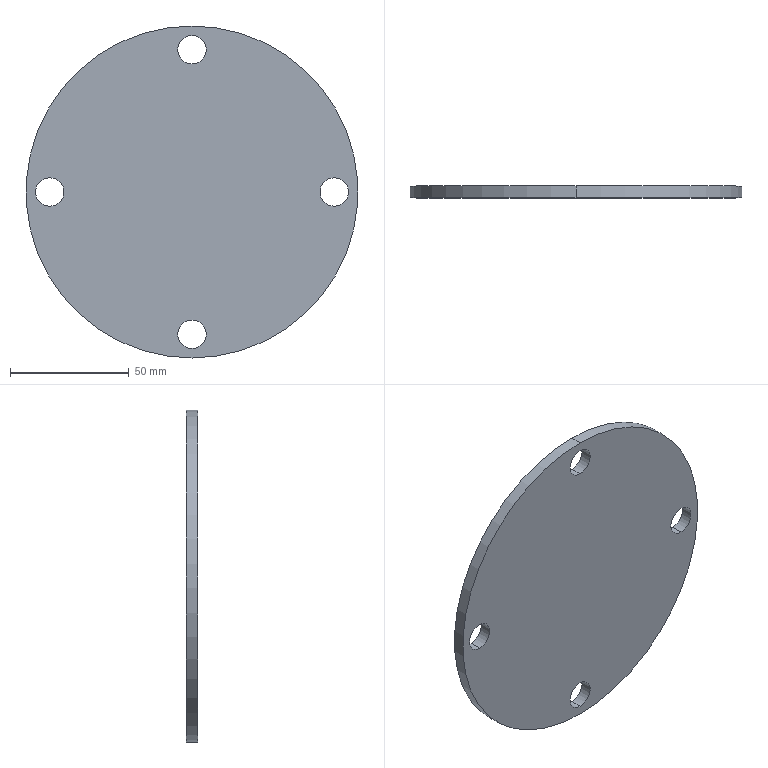Part | SolidWorks | features MirrorStock 1 | 1 solid | 12 faces | box 140 x 5 x 140 mm | volume 74707 mm3 | cylinder 10 | plane 2 | commonest cylinder face diameters 12 x8 140 x2
STEP:
#1=CARTESIAN_POINT('',(0.,0.,54.));
#2=VERTEX_POINT('',#1);
#3=CARTESIAN_POINT('',(0.,0.,66.));
#4=VERTEX_POINT('',#3);
#5=CARTESIAN_POINT('',(0.,0.,60.));
#6=DIRECTION('',(0.,-1.,0.));
#7=DIRECTION('',(0.,0.,-1.));
#8=AXIS2_PLACEMENT_3D('',#5,#6,#7);
#9=CIRCLE('',#8,6.);
#10=EDGE_CURVE('',#2,#4,#9,.T.);
#11=ORIENTED_EDGE('',*,*,#10,.T.);
#12=CARTESIAN_POINT('',(0.,5.,66.));
#13=VERTEX_POINT('',#12);
#14=CARTESIAN_POINT('',(0.,0.,66.));
#15=DIRECTION('',(0.,1.,0.));
#16=VECTOR('',#15,1000.);
#17=LINE('',#14,#16);
#18=EDGE_CURVE('',#4,#13,#17,.T.);
#19=ORIENTED_EDGE('',*,*,#18,.T.);
#20=CARTESIAN_POINT('',(0.,5.,54.));
#21=VERTEX_POINT('',#20);
#22=CARTESIAN_POINT('',(0.,5.,60.));
#23=DIRECTION('',(0.,-1.,0.));
#24=DIRECTION('',(0.,0.,-1.));
#25=AXIS2_PLACEMENT_3D('',#22,#23,#24);
#26=CIRCLE('',#25,6.);
#27=EDGE_CURVE('',#21,#13,#26,.T.);
#28=ORIENTED_EDGE('',*,*,#27,.F.);
#29=CARTESIAN_POINT('',(0.,0.,54.));
#30=DIRECTION('',(0.,1.,0.));
#31=VECTOR('',#30,1000.);
#32=LINE('',#29,#31);
#33=EDGE_CURVE('',#2,#21,#32,.T.);
#34=ORIENTED_EDGE('',*,*,#33,.F.);
#35=EDGE_LOOP('',(#11,#19,#28,#34));
#36=FACE_OUTER_BOUND('',#35,.T.);
#37=CARTESIAN_POINT('',(0.,0.,60.));
#38=DIRECTION('',(0.,1.,0.));
#39=DIRECTION('',(0.,0.,-1.));
#40=AXIS2_PLACEMENT_3D('',#37,#38,#39);
#41=CYLINDRICAL_SURFACE('',#40,6.);
#42=ADVANCED_FACE('',(#36),#41,.F.);
#43=CARTESIAN_POINT('',(60.,0.,-6.));
#44=VERTEX_POINT('',#43);
#45=CARTESIAN_POINT('',(60.,0.,6.));
#46=VERTEX_POINT('',#45);
#47=CARTESIAN_POINT('',(60.,0.,0.));
#48=DIRECTION('',(0.,-1.,0.));
#49=DIRECTION('',(0.,0.,-1.));
#50=AXIS2_PLACEMENT_3D('',#47,#48,#49);
#51=CIRCLE('',#50,6.);
#52=EDGE_CURVE('',#44,#46,#51,.T.);
#53=ORIENTED_EDGE('',*,*,#52,.T.);
#54=CARTESIAN_POINT('',(60.,5.,6.));
#55=VERTEX_POINT('',#54);
#56=CARTESIAN_POINT('',(60.,0.,6.));
#57=DIRECTION('',(0.,1.,0.));
#58=VECTOR('',#57,1000.);
#59=LINE('',#56,#58);
#60=EDGE_CURVE('',#46,#55,#59,.T.);
#61=ORIENTED_EDGE('',*,*,#60,.T.);
#62=CARTESIAN_POINT('',(60.,5.,-6.));
#63=VERTEX_POINT('',#62);
#64=CARTESIAN_POINT('',(60.,5.,0.));
#65=DIRECTION('',(0.,-1.,0.));
#66=DIRECTION('',(0.,0.,-1.));
#67=AXIS2_PLACEMENT_3D('',#64,#65,#66);
#68=CIRCLE('',#67,6.);
#69=EDGE_CURVE('',#63,#55,#68,.T.);
#70=ORIENTED_EDGE('',*,*,#69,.F.);
#71=CARTESIAN_POINT('',(60.,0.,-6.));
#72=DIRECTION('',(0.,1.,0.));
#73=VECTOR('',#72,1000.);
#74=LINE('',#71,#73);
#75=EDGE_CURVE('',#44,#63,#74,.T.);
#76=ORIENTED_EDGE('',*,*,#75,.F.);
#77=EDGE_LOOP('',(#53,#61,#70,#76));
#78=FACE_OUTER_BOUND('',#77,.T.);
#79=CARTESIAN_POINT('',(60.,0.,0.));
#80=DIRECTION('',(0.,1.,0.));
#81=DIRECTION('',(0.,0.,-1.));
#82=AXIS2_PLACEMENT_3D('',#79,#80,#81);
#83=CYLINDRICAL_SURFACE('',#82,6.);
#84=ADVANCED_FACE('',(#78),#83,.F.);
#85=CARTESIAN_POINT('',(0.,0.,-66.));
#86=VERTEX_POINT('',#85);
#87=CARTESIAN_POINT('',(0.,0.,-54.));
#88=VERTEX_POINT('',#87);
#89=CARTESIAN_POINT('',(0.,0.,-60.));
#90=DIRECTION('',(0.,-1.,0.));
#91=DIRECTION('',(0.,0.,-1.));
#92=AXIS2_PLACEMENT_3D('',#89,#90,#91);
#93=CIRCLE('',#92,6.);
#94=EDGE_CURVE('',#86,#88,#93,.T.);
#95=ORIENTED_EDGE('',*,*,#94,.T.);
#96=CARTESIAN_POINT('',(0.,5.,-54.));
#97=VERTEX_POINT('',#96);
#98=CARTESIAN_POINT('',(0.,0.,-54.));
#99=DIRECTION('',(0.,1.,0.));
#100=VECTOR('',#99,1000.);
#101=LINE('',#98,#100);
#102=EDGE_CURVE('',#88,#97,#101,.T.);
#103=ORIENTED_EDGE('',*,*,#102,.T.);
#104=CARTESIAN_POINT('',(0.,5.,-66.));
#105=VERTEX_POINT('',#104);
#106=CARTESIAN_POINT('',(0.,5.,-60.));
#107=DIRECTION('',(0.,-1.,0.));
#108=DIRECTION('',(0.,0.,-1.));
#109=AXIS2_PLACEMENT_3D('',#106,#107,#108);
#110=CIRCLE('',#109,6.);
#111=EDGE_CURVE('',#105,#97,#110,.T.);
#112=ORIENTED_EDGE('',*,*,#111,.F.);
#113=CARTESIAN_POINT('',(0.,0.,-66.));
#114=DIRECTION('',(0.,1.,0.));
#115=VECTOR('',#114,1000.);
#116=LINE('',#113,#115);
#117=EDGE_CURVE('',#86,#105,#116,.T.);
#118=ORIENTED_EDGE('',*,*,#117,.F.);
#119=EDGE_LOOP('',(#95,#103,#112,#118));
#120=FACE_OUTER_BOUND('',#119,.T.);
#121=CARTESIAN_POINT('',(0.,0.,-60.));
#122=DIRECTION('',(0.,1.,0.));
#123=DIRECTION('',(0.,0.,-1.));
#124=AXIS2_PLACEMENT_3D('',#121,#122,#123);
#125=CYLINDRICAL_SURFACE('',#124,6.);
#126=ADVANCED_FACE('',(#120),#125,.F.);
#127=CARTESIAN_POINT('',(-60.,0.,-6.));
#128=VERTEX_POINT('',#127);
#129=CARTESIAN_POINT('',(-60.,0.,6.));
#130=VERTEX_POINT('',#129);
#131=CARTESIAN_POINT('',(-60.,0.,0.));
#132=DIRECTION('',(0.,-1.,0.));
#133=DIRECTION('',(0.,0.,-1.));
#134=AXIS2_PLACEMENT_3D('',#131,#132,#133);
#135=CIRCLE('',#134,6.);
#136=EDGE_CURVE('',#128,#130,#135,.T.);
#137=ORIENTED_EDGE('',*,*,#136,.T.);
#138=CARTESIAN_POINT('',(-60.,5.,6.));
#139=VERTEX_POINT('',#138);
#140=CARTESIAN_POINT('',(-60.,0.,6.));
#141=DIRECTION('',(0.,1.,0.));
#142=VECTOR('',#141,1000.);
#143=LINE('',#140,#142);
#144=EDGE_CURVE('',#130,#139,#143,.T.);
#145=ORIENTED_EDGE('',*,*,#144,.T.);
#146=CARTESIAN_POINT('',(-60.,5.,-6.));
#147=VERTEX_POINT('',#146);
#148=CARTESIAN_POINT('',(-60.,5.,0.));
#149=DIRECTION('',(0.,-1.,0.));
#150=DIRECTION('',(0.,0.,-1.));
#151=AXIS2_PLACEMENT_3D('',#148,#149,#150);
#152=CIRCLE('',#151,6.);
#153=EDGE_CURVE('',#147,#139,#152,.T.);
#154=ORIENTED_EDGE('',*,*,#153,.F.);
#155=CARTESIAN_POINT('',(-60.,0.,-6.));
#156=DIRECTION('',(0.,1.,0.));
#157=VECTOR('',#156,1000.);
#158=LINE('',#155,#157);
#159=EDGE_CURVE('',#128,#147,#158,.T.);
#160=ORIENTED_EDGE('',*,*,#159,.F.);
#161=EDGE_LOOP('',(#137,#145,#154,#160));
#162=FACE_OUTER_BOUND('',#161,.T.);
#163=CARTESIAN_POINT('',(-60.,0.,0.));
#164=DIRECTION('',(0.,1.,0.));
#165=DIRECTION('',(0.,0.,-1.));
#166=AXIS2_PLACEMENT_3D('',#163,#164,#165);
#167=CYLINDRICAL_SURFACE('',#166,6.);
#168=ADVANCED_FACE('',(#162),#167,.F.);
#169=CARTESIAN_POINT('',(0.,5.,70.));
#170=VERTEX_POINT('',#169);
#171=CARTESIAN_POINT('',(0.,5.,-70.));
#172=VERTEX_POINT('',#171);
#173=CARTESIAN_POINT('',(0.,5.,0.));
#174=DIRECTION('',(0.,-1.,0.));
#175=DIRECTION('',(0.,0.,-1.));
#176=AXIS2_PLACEMENT_3D('',#173,#174,#175);
#177=CIRCLE('',#176,70.);
#178=EDGE_CURVE('',#170,#172,#177,.T.);
#179=ORIENTED_EDGE('',*,*,#178,.T.);
#180=CARTESIAN_POINT('',(0.,0.,-70.));
#181=VERTEX_POINT('',#180);
#182=CARTESIAN_POINT('',(0.,5.,-70.));
#183=DIRECTION('',(0.,-1.,0.));
#184=VECTOR('',#183,1000.);
#185=LINE('',#182,#184);
#186=EDGE_CURVE('',#172,#181,#185,.T.);
#187=ORIENTED_EDGE('',*,*,#186,.T.);
#188=CARTESIAN_POINT('',(0.,0.,70.));
#189=VERTEX_POINT('',#188);
#190=CARTESIAN_POINT('',(0.,0.,0.));
#191=DIRECTION('',(0.,-1.,0.));
#192=DIRECTION('',(0.,0.,-1.));
#193=AXIS2_PLACEMENT_3D('',#190,#191,#192);
#194=CIRCLE('',#193,70.);
#195=EDGE_CURVE('',#189,#181,#194,.T.);
#196=ORIENTED_EDGE('',*,*,#195,.F.);
#197=CARTESIAN_POINT('',(0.,5.,70.));
#198=DIRECTION('',(0.,-1.,0.));
#199=VECTOR('',#198,1000.);
#200=LINE('',#197,#199);
#201=EDGE_CURVE('',#170,#189,#200,.T.);
#202=ORIENTED_EDGE('',*,*,#201,.F.);
#203=EDGE_LOOP('',(#179,#187,#196,#202));
#204=FACE_OUTER_BOUND('',#203,.T.);
#205=CARTESIAN_POINT('',(0.,5.,0.));
#206=DIRECTION('',(0.,-1.,0.));
#207=DIRECTION('',(0.,0.,1.));
#208=AXIS2_PLACEMENT_3D('',#205,#206,#207);
#209=CYLINDRICAL_SURFACE('',#208,70.);
#210=ADVANCED_FACE('',(#204),#209,.T.);
#211=ORIENTED_EDGE('',*,*,#186,.F.);
#212=CARTESIAN_POINT('',(0.,5.,0.));
#213=DIRECTION('',(0.,-1.,0.));
#214=DIRECTION('',(0.,0.,-1.));
#215=AXIS2_PLACEMENT_3D('',#212,#213,#214);
#216=CIRCLE('',#215,70.);
#217=EDGE_CURVE('',#172,#170,#216,.T.);
#218=ORIENTED_EDGE('',*,*,#217,.T.);
#219=ORIENTED_EDGE('',*,*,#201,.T.);
#220=CARTESIAN_POINT('',(0.,0.,0.));
#221=DIRECTION('',(0.,-1.,0.));
#222=DIRECTION('',(0.,0.,-1.));
#223=AXIS2_PLACEMENT_3D('',#220,#221,#222);
#224=CIRCLE('',#223,70.);
#225=EDGE_CURVE('',#181,#189,#224,.T.);
#226=ORIENTED_EDGE('',*,*,#225,.F.);
#227=EDGE_LOOP('',(#211,#218,#219,#226));
#228=FACE_OUTER_BOUND('',#227,.T.);
#229=CARTESIAN_POINT('',(0.,5.,0.));
#230=DIRECTION('',(0.,-1.,0.));
#231=DIRECTION('',(0.,0.,1.));
#232=AXIS2_PLACEMENT_3D('',#229,#230,#231);
#233=CYLINDRICAL_SURFACE('',#232,70.);
#234=ADVANCED_FACE('',(#228),#233,.T.);
#235=ORIENTED_EDGE('',*,*,#27,.T.);
#236=CARTESIAN_POINT('',(0.,5.,60.));
#237=DIRECTION('',(0.,-1.,0.));
#238=DIRECTION('',(0.,0.,-1.));
#239=AXIS2_PLACEMENT_3D('',#236,#237,#238);
#240=CIRCLE('',#239,6.);
#241=EDGE_CURVE('',#13,#21,#240,.T.);
#242=ORIENTED_EDGE('',*,*,#241,.T.);
#243=EDGE_LOOP('',(#235,#242));
#244=FACE_BOUND('',#243,.T.);
#245=ORIENTED_EDGE('',*,*,#69,.T.);
#246=CARTESIAN_POINT('',(60.,5.,0.));
#247=DIRECTION('',(0.,-1.,0.));
#248=DIRECTION('',(0.,0.,-1.));
#249=AXIS2_PLACEMENT_3D('',#246,#247,#248);
#250=CIRCLE('',#249,6.);
#251=EDGE_CURVE('',#55,#63,#250,.T.);
#252=ORIENTED_EDGE('',*,*,#251,.T.);
#253=EDGE_LOOP('',(#245,#252));
#254=FACE_BOUND('',#253,.T.);
#255=ORIENTED_EDGE('',*,*,#111,.T.);
#256=CARTESIAN_POINT('',(0.,5.,-60.));
#257=DIRECTION('',(0.,-1.,0.));
#258=DIRECTION('',(0.,0.,-1.));
#259=AXIS2_PLACEMENT_3D('',#256,#257,#258);
#260=CIRCLE('',#259,6.);
#261=EDGE_CURVE('',#97,#105,#260,.T.);
#262=ORIENTED_EDGE('',*,*,#261,.T.);
#263=EDGE_LOOP('',(#255,#262));
#264=FACE_BOUND('',#263,.T.);
#265=ORIENTED_EDGE('',*,*,#153,.T.);
#266=CARTESIAN_POINT('',(-60.,5.,0.));
#267=DIRECTION('',(0.,-1.,0.));
#268=DIRECTION('',(0.,0.,-1.));
#269=AXIS2_PLACEMENT_3D('',#266,#267,#268);
#270=CIRCLE('',#269,6.);
#271=EDGE_CURVE('',#139,#147,#270,.T.);
#272=ORIENTED_EDGE('',*,*,#271,.T.);
#273=EDGE_LOOP('',(#265,#272));
#274=FACE_BOUND('',#273,.T.);
#275=ORIENTED_EDGE('',*,*,#178,.F.);
#276=ORIENTED_EDGE('',*,*,#217,.F.);
#277=EDGE_LOOP('',(#275,#276));
#278=FACE_OUTER_BOUND('',#277,.T.);
#279=CARTESIAN_POINT('',(0.,5.,0.));
#280=DIRECTION('',(0.,1.,0.));
#281=DIRECTION('',(0.,0.,-1.));
#282=AXIS2_PLACEMENT_3D('',#279,#280,#281);
#283=PLANE('',#282);
#284=ADVANCED_FACE('',(#244,#254,#264,#274,#278),#283,.T.);
#285=ORIENTED_EDGE('',*,*,#10,.F.);
#286=CARTESIAN_POINT('',(0.,0.,60.));
#287=DIRECTION('',(0.,-1.,0.));
#288=DIRECTION('',(0.,0.,-1.));
#289=AXIS2_PLACEMENT_3D('',#286,#287,#288);
#290=CIRCLE('',#289,6.);
#291=EDGE_CURVE('',#4,#2,#290,.T.);
#292=ORIENTED_EDGE('',*,*,#291,.F.);
#293=EDGE_LOOP('',(#285,#292));
#294=FACE_BOUND('',#293,.T.);
#295=ORIENTED_EDGE('',*,*,#52,.F.);
#296=CARTESIAN_POINT('',(60.,0.,0.));
#297=DIRECTION('',(0.,-1.,0.));
#298=DIRECTION('',(0.,0.,-1.));
#299=AXIS2_PLACEMENT_3D('',#296,#297,#298);
#300=CIRCLE('',#299,6.);
#301=EDGE_CURVE('',#46,#44,#300,.T.);
#302=ORIENTED_EDGE('',*,*,#301,.F.);
#303=EDGE_LOOP('',(#295,#302));
#304=FACE_BOUND('',#303,.T.);
#305=ORIENTED_EDGE('',*,*,#94,.F.);
#306=CARTESIAN_POINT('',(0.,0.,-60.));
#307=DIRECTION('',(0.,-1.,0.));
#308=DIRECTION('',(0.,0.,-1.));
#309=AXIS2_PLACEMENT_3D('',#306,#307,#308);
#310=CIRCLE('',#309,6.);
#311=EDGE_CURVE('',#88,#86,#310,.T.);
#312=ORIENTED_EDGE('',*,*,#311,.F.);
#313=EDGE_LOOP('',(#305,#312));
#314=FACE_BOUND('',#313,.T.);
#315=ORIENTED_EDGE('',*,*,#136,.F.);
#316=CARTESIAN_POINT('',(-60.,0.,0.));
#317=DIRECTION('',(0.,-1.,0.));
#318=DIRECTION('',(0.,0.,-1.));
#319=AXIS2_PLACEMENT_3D('',#316,#317,#318);
#320=CIRCLE('',#319,6.);
#321=EDGE_CURVE('',#130,#128,#320,.T.);
#322=ORIENTED_EDGE('',*,*,#321,.F.);
#323=EDGE_LOOP('',(#315,#322));
#324=FACE_BOUND('',#323,.T.);
#325=ORIENTED_EDGE('',*,*,#195,.T.);
#326=ORIENTED_EDGE('',*,*,#225,.T.);
#327=EDGE_LOOP('',(#325,#326));
#328=FACE_OUTER_BOUND('',#327,.T.);
#329=CARTESIAN_POINT('',(0.,0.,0.));
#330=DIRECTION('',(0.,1.,0.));
#331=DIRECTION('',(0.,0.,-1.));
#332=AXIS2_PLACEMENT_3D('',#329,#330,#331);
#333=PLANE('',#332);
#334=ADVANCED_FACE('',(#294,#304,#314,#324,#328),#333,.F.);
#335=ORIENTED_EDGE('',*,*,#144,.F.);
#336=ORIENTED_EDGE('',*,*,#321,.T.);
#337=ORIENTED_EDGE('',*,*,#159,.T.);
#338=ORIENTED_EDGE('',*,*,#271,.F.);
#339=EDGE_LOOP('',(#335,#336,#337,#338));
#340=FACE_OUTER_BOUND('',#339,.T.);
#341=CARTESIAN_POINT('',(-60.,0.,0.));
#342=DIRECTION('',(0.,1.,0.));
#343=DIRECTION('',(0.,0.,-1.));
#344=AXIS2_PLACEMENT_3D('',#341,#342,#343);
#345=CYLINDRICAL_SURFACE('',#344,6.);
#346=ADVANCED_FACE('',(#340),#345,.F.);
#347=ORIENTED_EDGE('',*,*,#102,.F.);
#348=ORIENTED_EDGE('',*,*,#311,.T.);
#349=ORIENTED_EDGE('',*,*,#117,.T.);
#350=ORIENTED_EDGE('',*,*,#261,.F.);
#351=EDGE_LOOP('',(#347,#348,#349,#350));
#352=FACE_OUTER_BOUND('',#351,.T.);
#353=CARTESIAN_POINT('',(0.,0.,-60.));
#354=DIRECTION('',(0.,1.,0.));
#355=DIRECTION('',(0.,0.,-1.));
#356=AXIS2_PLACEMENT_3D('',#353,#354,#355);
#357=CYLINDRICAL_SURFACE('',#356,6.);
#358=ADVANCED_FACE('',(#352),#357,.F.);
#359=ORIENTED_EDGE('',*,*,#60,.F.);
#360=ORIENTED_EDGE('',*,*,#301,.T.);
#361=ORIENTED_EDGE('',*,*,#75,.T.);
#362=ORIENTED_EDGE('',*,*,#251,.F.);
#363=EDGE_LOOP('',(#359,#360,#361,#362));
#364=FACE_OUTER_BOUND('',#363,.T.);
#365=CARTESIAN_POINT('',(60.,0.,0.));
#366=DIRECTION('',(0.,1.,0.));
#367=DIRECTION('',(0.,0.,-1.));
#368=AXIS2_PLACEMENT_3D('',#365,#366,#367);
#369=CYLINDRICAL_SURFACE('',#368,6.);
#370=ADVANCED_FACE('',(#364),#369,.F.);
#371=ORIENTED_EDGE('',*,*,#18,.F.);
#372=ORIENTED_EDGE('',*,*,#291,.T.);
#373=ORIENTED_EDGE('',*,*,#33,.T.);
#374=ORIENTED_EDGE('',*,*,#241,.F.);
#375=EDGE_LOOP('',(#371,#372,#373,#374));
#376=FACE_OUTER_BOUND('',#375,.T.);
#377=CARTESIAN_POINT('',(0.,0.,60.));
#378=DIRECTION('',(0.,1.,0.));
#379=DIRECTION('',(0.,0.,-1.));
#380=AXIS2_PLACEMENT_3D('',#377,#378,#379);
#381=CYLINDRICAL_SURFACE('',#380,6.);
#382=ADVANCED_FACE('',(#376),#381,.F.);
#383=CLOSED_SHELL('',(#42,#84,#126,#168,#210,#234,#284,#334,#346,#358,#370,#382));
#384=MANIFOLD_SOLID_BREP('',#383);
#385=CARTESIAN_POINT('',(0.,0.,0.));
#386=DIRECTION('',(0.,0.,1.));
#387=DIRECTION('',(1.,0.,0.));
#388=AXIS2_PLACEMENT_3D('',#385,#386,#387);
#389=(LENGTH_UNIT()NAMED_UNIT(*)SI_UNIT(.MILLI.,.METRE.));
#390=UNCERTAINTY_MEASURE_WITH_UNIT(LENGTH_MEASURE(0.00001),#389,'','');
#391=(NAMED_UNIT(*)PLANE_ANGLE_UNIT()SI_UNIT($,.RADIAN.));
#392=(NAMED_UNIT(*)SI_UNIT($,.STERADIAN.)SOLID_ANGLE_UNIT());
#393=(GEOMETRIC_REPRESENTATION_CONTEXT(3)GLOBAL_UNCERTAINTY_ASSIGNED_CONTEXT((#390))GLOBAL_UNIT_ASSIGNED_CONTEXT((#389,#391,#392))REPRESENTATION_CONTEXT('',''));
#394=ADVANCED_BREP_SHAPE_REPRESENTATION('',(#384,#388),#393);